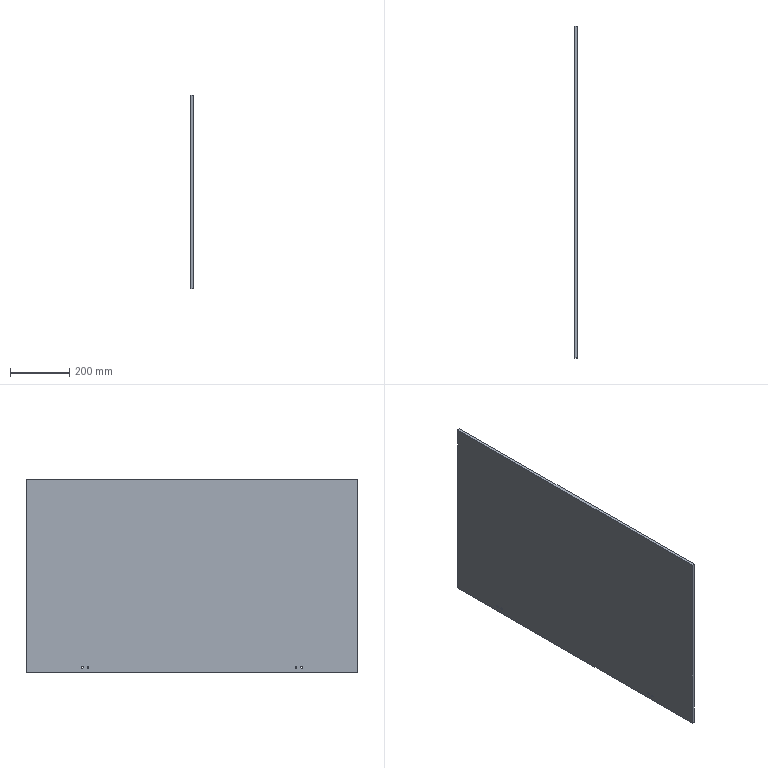Part | 1 solid | 14 faces | box 10 x 1121 x 654 mm | volume 7330209 mm3 | cylinder 8 | plane 6 | commonest cylinder face diameters 6 x8
STEP:
#1=CARTESIAN_POINT('',(10.,370.5,-306.));
#2=VERTEX_POINT('',#1);
#3=CARTESIAN_POINT('',(10.,370.5,-312.));
#4=VERTEX_POINT('',#3);
#5=CARTESIAN_POINT('',(10.,370.5,-309.));
#6=DIRECTION('',(1.,0.,0.));
#7=DIRECTION('',(0.,0.,-1.));
#8=AXIS2_PLACEMENT_3D('',#5,#6,#7);
#9=CIRCLE('',#8,3.);
#10=EDGE_CURVE('',#2,#4,#9,.T.);
#11=ORIENTED_EDGE('',*,*,#10,.T.);
#12=CARTESIAN_POINT('',(0.,370.5,-312.));
#13=VERTEX_POINT('',#12);
#14=CARTESIAN_POINT('',(10.,370.5,-312.));
#15=DIRECTION('',(-1.,0.,0.));
#16=VECTOR('',#15,1000.);
#17=LINE('',#14,#16);
#18=EDGE_CURVE('',#4,#13,#17,.T.);
#19=ORIENTED_EDGE('',*,*,#18,.T.);
#20=CARTESIAN_POINT('',(0.,370.5,-306.));
#21=VERTEX_POINT('',#20);
#22=CARTESIAN_POINT('',(0.,370.5,-309.));
#23=DIRECTION('',(1.,0.,0.));
#24=DIRECTION('',(0.,0.,-1.));
#25=AXIS2_PLACEMENT_3D('',#22,#23,#24);
#26=CIRCLE('',#25,3.);
#27=EDGE_CURVE('',#21,#13,#26,.T.);
#28=ORIENTED_EDGE('',*,*,#27,.F.);
#29=CARTESIAN_POINT('',(10.,370.5,-306.));
#30=DIRECTION('',(-1.,0.,0.));
#31=VECTOR('',#30,1000.);
#32=LINE('',#29,#31);
#33=EDGE_CURVE('',#2,#21,#32,.T.);
#34=ORIENTED_EDGE('',*,*,#33,.F.);
#35=EDGE_LOOP('',(#11,#19,#28,#34));
#36=FACE_OUTER_BOUND('',#35,.T.);
#37=CARTESIAN_POINT('',(10.,370.5,-309.));
#38=DIRECTION('',(-1.,0.,0.));
#39=DIRECTION('',(0.,0.,1.));
#40=AXIS2_PLACEMENT_3D('',#37,#38,#39);
#41=CYLINDRICAL_SURFACE('',#40,3.);
#42=ADVANCED_FACE('',(#36),#41,.F.);
#43=CARTESIAN_POINT('',(10.,351.5,-306.));
#44=VERTEX_POINT('',#43);
#45=CARTESIAN_POINT('',(10.,351.5,-312.));
#46=VERTEX_POINT('',#45);
#47=CARTESIAN_POINT('',(10.,351.5,-309.));
#48=DIRECTION('',(1.,0.,0.));
#49=DIRECTION('',(0.,0.,-1.));
#50=AXIS2_PLACEMENT_3D('',#47,#48,#49);
#51=CIRCLE('',#50,3.);
#52=EDGE_CURVE('',#44,#46,#51,.T.);
#53=ORIENTED_EDGE('',*,*,#52,.T.);
#54=CARTESIAN_POINT('',(0.,351.5,-312.));
#55=VERTEX_POINT('',#54);
#56=CARTESIAN_POINT('',(10.,351.5,-312.));
#57=DIRECTION('',(-1.,0.,0.));
#58=VECTOR('',#57,1000.);
#59=LINE('',#56,#58);
#60=EDGE_CURVE('',#46,#55,#59,.T.);
#61=ORIENTED_EDGE('',*,*,#60,.T.);
#62=CARTESIAN_POINT('',(0.,351.5,-306.));
#63=VERTEX_POINT('',#62);
#64=CARTESIAN_POINT('',(0.,351.5,-309.));
#65=DIRECTION('',(1.,0.,0.));
#66=DIRECTION('',(0.,0.,-1.));
#67=AXIS2_PLACEMENT_3D('',#64,#65,#66);
#68=CIRCLE('',#67,3.);
#69=EDGE_CURVE('',#63,#55,#68,.T.);
#70=ORIENTED_EDGE('',*,*,#69,.F.);
#71=CARTESIAN_POINT('',(10.,351.5,-306.));
#72=DIRECTION('',(-1.,0.,0.));
#73=VECTOR('',#72,1000.);
#74=LINE('',#71,#73);
#75=EDGE_CURVE('',#44,#63,#74,.T.);
#76=ORIENTED_EDGE('',*,*,#75,.F.);
#77=EDGE_LOOP('',(#53,#61,#70,#76));
#78=FACE_OUTER_BOUND('',#77,.T.);
#79=CARTESIAN_POINT('',(10.,351.5,-309.));
#80=DIRECTION('',(-1.,0.,0.));
#81=DIRECTION('',(0.,0.,1.));
#82=AXIS2_PLACEMENT_3D('',#79,#80,#81);
#83=CYLINDRICAL_SURFACE('',#82,3.);
#84=ADVANCED_FACE('',(#78),#83,.F.);
#85=CARTESIAN_POINT('',(10.,-370.5,-312.));
#86=VERTEX_POINT('',#85);
#87=CARTESIAN_POINT('',(10.,-370.5,-306.));
#88=VERTEX_POINT('',#87);
#89=CARTESIAN_POINT('',(10.,-370.5,-309.));
#90=DIRECTION('',(-1.,0.,0.));
#91=DIRECTION('',(0.,0.,-1.));
#92=AXIS2_PLACEMENT_3D('',#89,#90,#91);
#93=CIRCLE('',#92,3.);
#94=EDGE_CURVE('',#86,#88,#93,.T.);
#95=ORIENTED_EDGE('',*,*,#94,.F.);
#96=CARTESIAN_POINT('',(0.,-370.5,-312.));
#97=VERTEX_POINT('',#96);
#98=CARTESIAN_POINT('',(10.,-370.5,-312.));
#99=DIRECTION('',(-1.,0.,0.));
#100=VECTOR('',#99,1000.);
#101=LINE('',#98,#100);
#102=EDGE_CURVE('',#86,#97,#101,.T.);
#103=ORIENTED_EDGE('',*,*,#102,.T.);
#104=CARTESIAN_POINT('',(0.,-370.5,-306.));
#105=VERTEX_POINT('',#104);
#106=CARTESIAN_POINT('',(0.,-370.5,-309.));
#107=DIRECTION('',(-1.,0.,0.));
#108=DIRECTION('',(0.,0.,-1.));
#109=AXIS2_PLACEMENT_3D('',#106,#107,#108);
#110=CIRCLE('',#109,3.);
#111=EDGE_CURVE('',#97,#105,#110,.T.);
#112=ORIENTED_EDGE('',*,*,#111,.T.);
#113=CARTESIAN_POINT('',(10.,-370.5,-306.));
#114=DIRECTION('',(-1.,0.,0.));
#115=VECTOR('',#114,1000.);
#116=LINE('',#113,#115);
#117=EDGE_CURVE('',#88,#105,#116,.T.);
#118=ORIENTED_EDGE('',*,*,#117,.F.);
#119=EDGE_LOOP('',(#95,#103,#112,#118));
#120=FACE_OUTER_BOUND('',#119,.T.);
#121=CARTESIAN_POINT('',(10.,-370.5,-309.));
#122=DIRECTION('',(-1.,0.,0.));
#123=DIRECTION('',(0.,0.,1.));
#124=AXIS2_PLACEMENT_3D('',#121,#122,#123);
#125=CYLINDRICAL_SURFACE('',#124,3.);
#126=ADVANCED_FACE('',(#120),#125,.F.);
#127=CARTESIAN_POINT('',(10.,-351.5,-312.));
#128=VERTEX_POINT('',#127);
#129=CARTESIAN_POINT('',(10.,-351.5,-306.));
#130=VERTEX_POINT('',#129);
#131=CARTESIAN_POINT('',(10.,-351.5,-309.));
#132=DIRECTION('',(-1.,0.,0.));
#133=DIRECTION('',(0.,0.,-1.));
#134=AXIS2_PLACEMENT_3D('',#131,#132,#133);
#135=CIRCLE('',#134,3.);
#136=EDGE_CURVE('',#128,#130,#135,.T.);
#137=ORIENTED_EDGE('',*,*,#136,.F.);
#138=CARTESIAN_POINT('',(0.,-351.5,-312.));
#139=VERTEX_POINT('',#138);
#140=CARTESIAN_POINT('',(10.,-351.5,-312.));
#141=DIRECTION('',(-1.,0.,0.));
#142=VECTOR('',#141,1000.);
#143=LINE('',#140,#142);
#144=EDGE_CURVE('',#128,#139,#143,.T.);
#145=ORIENTED_EDGE('',*,*,#144,.T.);
#146=CARTESIAN_POINT('',(0.,-351.5,-306.));
#147=VERTEX_POINT('',#146);
#148=CARTESIAN_POINT('',(0.,-351.5,-309.));
#149=DIRECTION('',(-1.,0.,0.));
#150=DIRECTION('',(0.,0.,-1.));
#151=AXIS2_PLACEMENT_3D('',#148,#149,#150);
#152=CIRCLE('',#151,3.);
#153=EDGE_CURVE('',#139,#147,#152,.T.);
#154=ORIENTED_EDGE('',*,*,#153,.T.);
#155=CARTESIAN_POINT('',(10.,-351.5,-306.));
#156=DIRECTION('',(-1.,0.,0.));
#157=VECTOR('',#156,1000.);
#158=LINE('',#155,#157);
#159=EDGE_CURVE('',#130,#147,#158,.T.);
#160=ORIENTED_EDGE('',*,*,#159,.F.);
#161=EDGE_LOOP('',(#137,#145,#154,#160));
#162=FACE_OUTER_BOUND('',#161,.T.);
#163=CARTESIAN_POINT('',(10.,-351.5,-309.));
#164=DIRECTION('',(-1.,0.,0.));
#165=DIRECTION('',(0.,0.,1.));
#166=AXIS2_PLACEMENT_3D('',#163,#164,#165);
#167=CYLINDRICAL_SURFACE('',#166,3.);
#168=ADVANCED_FACE('',(#162),#167,.F.);
#169=ORIENTED_EDGE('',*,*,#52,.F.);
#170=CARTESIAN_POINT('',(10.,351.5,-309.));
#171=DIRECTION('',(1.,0.,0.));
#172=DIRECTION('',(0.,0.,-1.));
#173=AXIS2_PLACEMENT_3D('',#170,#171,#172);
#174=CIRCLE('',#173,3.);
#175=EDGE_CURVE('',#46,#44,#174,.T.);
#176=ORIENTED_EDGE('',*,*,#175,.F.);
#177=EDGE_LOOP('',(#169,#176));
#178=FACE_BOUND('',#177,.T.);
#179=CARTESIAN_POINT('',(10.,-370.5,-309.));
#180=DIRECTION('',(-1.,0.,0.));
#181=DIRECTION('',(0.,0.,-1.));
#182=AXIS2_PLACEMENT_3D('',#179,#180,#181);
#183=CIRCLE('',#182,3.);
#184=EDGE_CURVE('',#88,#86,#183,.T.);
#185=ORIENTED_EDGE('',*,*,#184,.T.);
#186=ORIENTED_EDGE('',*,*,#94,.T.);
#187=EDGE_LOOP('',(#185,#186));
#188=FACE_BOUND('',#187,.T.);
#189=CARTESIAN_POINT('',(10.,-351.5,-309.));
#190=DIRECTION('',(-1.,0.,0.));
#191=DIRECTION('',(0.,0.,-1.));
#192=AXIS2_PLACEMENT_3D('',#189,#190,#191);
#193=CIRCLE('',#192,3.);
#194=EDGE_CURVE('',#130,#128,#193,.T.);
#195=ORIENTED_EDGE('',*,*,#194,.T.);
#196=ORIENTED_EDGE('',*,*,#136,.T.);
#197=EDGE_LOOP('',(#195,#196));
#198=FACE_BOUND('',#197,.T.);
#199=CARTESIAN_POINT('',(10.,-560.5,-327.));
#200=VERTEX_POINT('',#199);
#201=CARTESIAN_POINT('',(10.,560.5,-327.));
#202=VERTEX_POINT('',#201);
#203=CARTESIAN_POINT('',(10.,560.5,-327.));
#204=DIRECTION('',(0.,1.,0.));
#205=VECTOR('',#204,1000.);
#206=LINE('',#203,#205);
#207=EDGE_CURVE('',#200,#202,#206,.T.);
#208=ORIENTED_EDGE('',*,*,#207,.T.);
#209=CARTESIAN_POINT('',(10.,560.5,327.));
#210=VERTEX_POINT('',#209);
#211=CARTESIAN_POINT('',(10.,560.5,327.));
#212=DIRECTION('',(0.,0.,1.));
#213=VECTOR('',#212,1000.);
#214=LINE('',#211,#213);
#215=EDGE_CURVE('',#202,#210,#214,.T.);
#216=ORIENTED_EDGE('',*,*,#215,.T.);
#217=CARTESIAN_POINT('',(10.,-560.5,327.));
#218=VERTEX_POINT('',#217);
#219=CARTESIAN_POINT('',(10.,560.5,327.));
#220=DIRECTION('',(0.,-1.,0.));
#221=VECTOR('',#220,1000.);
#222=LINE('',#219,#221);
#223=EDGE_CURVE('',#210,#218,#222,.T.);
#224=ORIENTED_EDGE('',*,*,#223,.T.);
#225=CARTESIAN_POINT('',(10.,-560.5,327.));
#226=DIRECTION('',(0.,0.,-1.));
#227=VECTOR('',#226,1000.);
#228=LINE('',#225,#227);
#229=EDGE_CURVE('',#218,#200,#228,.T.);
#230=ORIENTED_EDGE('',*,*,#229,.T.);
#231=EDGE_LOOP('',(#208,#216,#224,#230));
#232=FACE_OUTER_BOUND('',#231,.T.);
#233=ORIENTED_EDGE('',*,*,#10,.F.);
#234=CARTESIAN_POINT('',(10.,370.5,-309.));
#235=DIRECTION('',(1.,0.,0.));
#236=DIRECTION('',(0.,0.,-1.));
#237=AXIS2_PLACEMENT_3D('',#234,#235,#236);
#238=CIRCLE('',#237,3.);
#239=EDGE_CURVE('',#4,#2,#238,.T.);
#240=ORIENTED_EDGE('',*,*,#239,.F.);
#241=EDGE_LOOP('',(#233,#240));
#242=FACE_BOUND('',#241,.T.);
#243=CARTESIAN_POINT('',(10.,0.,0.));
#244=DIRECTION('',(1.,0.,0.));
#245=DIRECTION('',(0.,0.,-1.));
#246=AXIS2_PLACEMENT_3D('',#243,#244,#245);
#247=PLANE('',#246);
#248=ADVANCED_FACE('',(#178,#188,#198,#232,#242),#247,.T.);
#249=CARTESIAN_POINT('',(0.,-370.5,-309.));
#250=DIRECTION('',(-1.,0.,0.));
#251=DIRECTION('',(0.,0.,-1.));
#252=AXIS2_PLACEMENT_3D('',#249,#250,#251);
#253=CIRCLE('',#252,3.);
#254=EDGE_CURVE('',#105,#97,#253,.T.);
#255=ORIENTED_EDGE('',*,*,#254,.F.);
#256=ORIENTED_EDGE('',*,*,#111,.F.);
#257=EDGE_LOOP('',(#255,#256));
#258=FACE_BOUND('',#257,.T.);
#259=CARTESIAN_POINT('',(0.,-351.5,-309.));
#260=DIRECTION('',(-1.,0.,0.));
#261=DIRECTION('',(0.,0.,-1.));
#262=AXIS2_PLACEMENT_3D('',#259,#260,#261);
#263=CIRCLE('',#262,3.);
#264=EDGE_CURVE('',#147,#139,#263,.T.);
#265=ORIENTED_EDGE('',*,*,#264,.F.);
#266=ORIENTED_EDGE('',*,*,#153,.F.);
#267=EDGE_LOOP('',(#265,#266));
#268=FACE_BOUND('',#267,.T.);
#269=CARTESIAN_POINT('',(0.,-560.5,-327.));
#270=VERTEX_POINT('',#269);
#271=CARTESIAN_POINT('',(0.,560.5,-327.));
#272=VERTEX_POINT('',#271);
#273=CARTESIAN_POINT('',(0.,560.5,-327.));
#274=DIRECTION('',(0.,1.,0.));
#275=VECTOR('',#274,1000.);
#276=LINE('',#273,#275);
#277=EDGE_CURVE('',#270,#272,#276,.T.);
#278=ORIENTED_EDGE('',*,*,#277,.F.);
#279=CARTESIAN_POINT('',(0.,-560.5,327.));
#280=VERTEX_POINT('',#279);
#281=CARTESIAN_POINT('',(0.,-560.5,327.));
#282=DIRECTION('',(0.,0.,-1.));
#283=VECTOR('',#282,1000.);
#284=LINE('',#281,#283);
#285=EDGE_CURVE('',#280,#270,#284,.T.);
#286=ORIENTED_EDGE('',*,*,#285,.F.);
#287=CARTESIAN_POINT('',(0.,560.5,327.));
#288=VERTEX_POINT('',#287);
#289=CARTESIAN_POINT('',(0.,560.5,327.));
#290=DIRECTION('',(0.,-1.,0.));
#291=VECTOR('',#290,1000.);
#292=LINE('',#289,#291);
#293=EDGE_CURVE('',#288,#280,#292,.T.);
#294=ORIENTED_EDGE('',*,*,#293,.F.);
#295=CARTESIAN_POINT('',(0.,560.5,327.));
#296=DIRECTION('',(0.,0.,1.));
#297=VECTOR('',#296,1000.);
#298=LINE('',#295,#297);
#299=EDGE_CURVE('',#272,#288,#298,.T.);
#300=ORIENTED_EDGE('',*,*,#299,.F.);
#301=EDGE_LOOP('',(#278,#286,#294,#300));
#302=FACE_OUTER_BOUND('',#301,.T.);
#303=ORIENTED_EDGE('',*,*,#69,.T.);
#304=CARTESIAN_POINT('',(0.,351.5,-309.));
#305=DIRECTION('',(1.,0.,0.));
#306=DIRECTION('',(0.,0.,-1.));
#307=AXIS2_PLACEMENT_3D('',#304,#305,#306);
#308=CIRCLE('',#307,3.);
#309=EDGE_CURVE('',#55,#63,#308,.T.);
#310=ORIENTED_EDGE('',*,*,#309,.T.);
#311=EDGE_LOOP('',(#303,#310));
#312=FACE_BOUND('',#311,.T.);
#313=ORIENTED_EDGE('',*,*,#27,.T.);
#314=CARTESIAN_POINT('',(0.,370.5,-309.));
#315=DIRECTION('',(1.,0.,0.));
#316=DIRECTION('',(0.,0.,-1.));
#317=AXIS2_PLACEMENT_3D('',#314,#315,#316);
#318=CIRCLE('',#317,3.);
#319=EDGE_CURVE('',#13,#21,#318,.T.);
#320=ORIENTED_EDGE('',*,*,#319,.T.);
#321=EDGE_LOOP('',(#313,#320));
#322=FACE_BOUND('',#321,.T.);
#323=CARTESIAN_POINT('',(0.,0.,0.));
#324=DIRECTION('',(1.,0.,0.));
#325=DIRECTION('',(0.,0.,-1.));
#326=AXIS2_PLACEMENT_3D('',#323,#324,#325);
#327=PLANE('',#326);
#328=ADVANCED_FACE('',(#258,#268,#302,#312,#322),#327,.F.);
#329=ORIENTED_EDGE('',*,*,#277,.T.);
#330=CARTESIAN_POINT('',(10.,560.5,-327.));
#331=DIRECTION('',(-1.,0.,0.));
#332=VECTOR('',#331,1000.);
#333=LINE('',#330,#332);
#334=EDGE_CURVE('',#202,#272,#333,.T.);
#335=ORIENTED_EDGE('',*,*,#334,.F.);
#336=ORIENTED_EDGE('',*,*,#207,.F.);
#337=CARTESIAN_POINT('',(10.,-560.5,-327.));
#338=DIRECTION('',(-1.,0.,0.));
#339=VECTOR('',#338,1000.);
#340=LINE('',#337,#339);
#341=EDGE_CURVE('',#200,#270,#340,.T.);
#342=ORIENTED_EDGE('',*,*,#341,.T.);
#343=EDGE_LOOP('',(#329,#335,#336,#342));
#344=FACE_OUTER_BOUND('',#343,.T.);
#345=CARTESIAN_POINT('',(10.,560.5,-327.));
#346=DIRECTION('',(0.,0.,1.));
#347=DIRECTION('',(0.,-1.,0.));
#348=AXIS2_PLACEMENT_3D('',#345,#346,#347);
#349=PLANE('',#348);
#350=ADVANCED_FACE('',(#344),#349,.F.);
#351=ORIENTED_EDGE('',*,*,#299,.T.);
#352=CARTESIAN_POINT('',(10.,560.5,327.));
#353=DIRECTION('',(-1.,0.,0.));
#354=VECTOR('',#353,1000.);
#355=LINE('',#352,#354);
#356=EDGE_CURVE('',#210,#288,#355,.T.);
#357=ORIENTED_EDGE('',*,*,#356,.F.);
#358=ORIENTED_EDGE('',*,*,#215,.F.);
#359=ORIENTED_EDGE('',*,*,#334,.T.);
#360=EDGE_LOOP('',(#351,#357,#358,#359));
#361=FACE_OUTER_BOUND('',#360,.T.);
#362=CARTESIAN_POINT('',(10.,560.5,327.));
#363=DIRECTION('',(0.,-1.,0.));
#364=DIRECTION('',(0.,0.,-1.));
#365=AXIS2_PLACEMENT_3D('',#362,#363,#364);
#366=PLANE('',#365);
#367=ADVANCED_FACE('',(#361),#366,.F.);
#368=ORIENTED_EDGE('',*,*,#293,.T.);
#369=CARTESIAN_POINT('',(10.,-560.5,327.));
#370=DIRECTION('',(-1.,0.,0.));
#371=VECTOR('',#370,1000.);
#372=LINE('',#369,#371);
#373=EDGE_CURVE('',#218,#280,#372,.T.);
#374=ORIENTED_EDGE('',*,*,#373,.F.);
#375=ORIENTED_EDGE('',*,*,#223,.F.);
#376=ORIENTED_EDGE('',*,*,#356,.T.);
#377=EDGE_LOOP('',(#368,#374,#375,#376));
#378=FACE_OUTER_BOUND('',#377,.T.);
#379=CARTESIAN_POINT('',(10.,560.5,327.));
#380=DIRECTION('',(0.,0.,-1.));
#381=DIRECTION('',(0.,1.,0.));
#382=AXIS2_PLACEMENT_3D('',#379,#380,#381);
#383=PLANE('',#382);
#384=ADVANCED_FACE('',(#378),#383,.F.);
#385=ORIENTED_EDGE('',*,*,#285,.T.);
#386=ORIENTED_EDGE('',*,*,#341,.F.);
#387=ORIENTED_EDGE('',*,*,#229,.F.);
#388=ORIENTED_EDGE('',*,*,#373,.T.);
#389=EDGE_LOOP('',(#385,#386,#387,#388));
#390=FACE_OUTER_BOUND('',#389,.T.);
#391=CARTESIAN_POINT('',(10.,-560.5,327.));
#392=DIRECTION('',(0.,1.,0.));
#393=DIRECTION('',(0.,0.,1.));
#394=AXIS2_PLACEMENT_3D('',#391,#392,#393);
#395=PLANE('',#394);
#396=ADVANCED_FACE('',(#390),#395,.F.);
#397=ORIENTED_EDGE('',*,*,#144,.F.);
#398=ORIENTED_EDGE('',*,*,#194,.F.);
#399=ORIENTED_EDGE('',*,*,#159,.T.);
#400=ORIENTED_EDGE('',*,*,#264,.T.);
#401=EDGE_LOOP('',(#397,#398,#399,#400));
#402=FACE_OUTER_BOUND('',#401,.T.);
#403=CARTESIAN_POINT('',(10.,-351.5,-309.));
#404=DIRECTION('',(-1.,0.,0.));
#405=DIRECTION('',(0.,0.,1.));
#406=AXIS2_PLACEMENT_3D('',#403,#404,#405);
#407=CYLINDRICAL_SURFACE('',#406,3.);
#408=ADVANCED_FACE('',(#402),#407,.F.);
#409=ORIENTED_EDGE('',*,*,#102,.F.);
#410=ORIENTED_EDGE('',*,*,#184,.F.);
#411=ORIENTED_EDGE('',*,*,#117,.T.);
#412=ORIENTED_EDGE('',*,*,#254,.T.);
#413=EDGE_LOOP('',(#409,#410,#411,#412));
#414=FACE_OUTER_BOUND('',#413,.T.);
#415=CARTESIAN_POINT('',(10.,-370.5,-309.));
#416=DIRECTION('',(-1.,0.,0.));
#417=DIRECTION('',(0.,0.,1.));
#418=AXIS2_PLACEMENT_3D('',#415,#416,#417);
#419=CYLINDRICAL_SURFACE('',#418,3.);
#420=ADVANCED_FACE('',(#414),#419,.F.);
#421=ORIENTED_EDGE('',*,*,#60,.F.);
#422=ORIENTED_EDGE('',*,*,#175,.T.);
#423=ORIENTED_EDGE('',*,*,#75,.T.);
#424=ORIENTED_EDGE('',*,*,#309,.F.);
#425=EDGE_LOOP('',(#421,#422,#423,#424));
#426=FACE_OUTER_BOUND('',#425,.T.);
#427=CARTESIAN_POINT('',(10.,351.5,-309.));
#428=DIRECTION('',(-1.,0.,0.));
#429=DIRECTION('',(0.,0.,1.));
#430=AXIS2_PLACEMENT_3D('',#427,#428,#429);
#431=CYLINDRICAL_SURFACE('',#430,3.);
#432=ADVANCED_FACE('',(#426),#431,.F.);
#433=ORIENTED_EDGE('',*,*,#18,.F.);
#434=ORIENTED_EDGE('',*,*,#239,.T.);
#435=ORIENTED_EDGE('',*,*,#33,.T.);
#436=ORIENTED_EDGE('',*,*,#319,.F.);
#437=EDGE_LOOP('',(#433,#434,#435,#436));
#438=FACE_OUTER_BOUND('',#437,.T.);
#439=CARTESIAN_POINT('',(10.,370.5,-309.));
#440=DIRECTION('',(-1.,0.,0.));
#441=DIRECTION('',(0.,0.,1.));
#442=AXIS2_PLACEMENT_3D('',#439,#440,#441);
#443=CYLINDRICAL_SURFACE('',#442,3.);
#444=ADVANCED_FACE('',(#438),#443,.F.);
#445=CLOSED_SHELL('',(#42,#84,#126,#168,#248,#328,#350,#367,#384,#396,#408,#420,#432,#444));
#446=MANIFOLD_SOLID_BREP('',#445);
#447=CARTESIAN_POINT('',(0.,0.,0.));
#448=DIRECTION('',(0.,0.,1.));
#449=DIRECTION('',(1.,0.,0.));
#450=AXIS2_PLACEMENT_3D('',#447,#448,#449);
#451=(LENGTH_UNIT()NAMED_UNIT(*)SI_UNIT(.MILLI.,.METRE.));
#452=UNCERTAINTY_MEASURE_WITH_UNIT(LENGTH_MEASURE(0.00001),#451,'','');
#453=(NAMED_UNIT(*)PLANE_ANGLE_UNIT()SI_UNIT($,.RADIAN.));
#454=(NAMED_UNIT(*)SI_UNIT($,.STERADIAN.)SOLID_ANGLE_UNIT());
#455=(GEOMETRIC_REPRESENTATION_CONTEXT(3)GLOBAL_UNCERTAINTY_ASSIGNED_CONTEXT((#452))GLOBAL_UNIT_ASSIGNED_CONTEXT((#451,#453,#454))REPRESENTATION_CONTEXT('',''));
#456=ADVANCED_BREP_SHAPE_REPRESENTATION('',(#446,#450),#455);